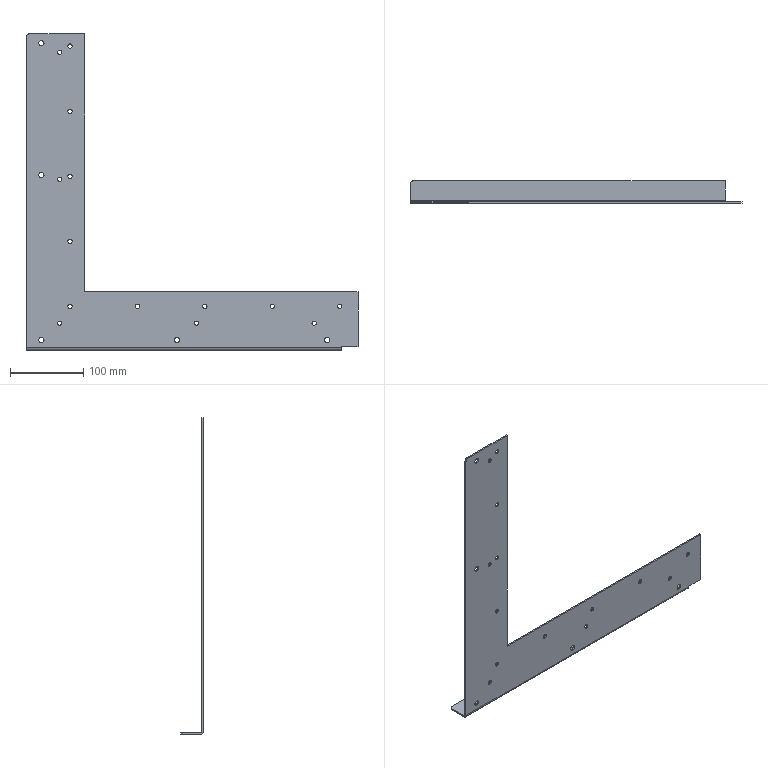Part | NX | features solid 2 | 1 solid | 54 faces | box 452.999 x 31 x 432 mm | volume 151182 mm3 | cylinder 42 | plane 12 | commonest cylinder face diameters 6 x28 7.2 x10 10 x2 4 x1 8 x1